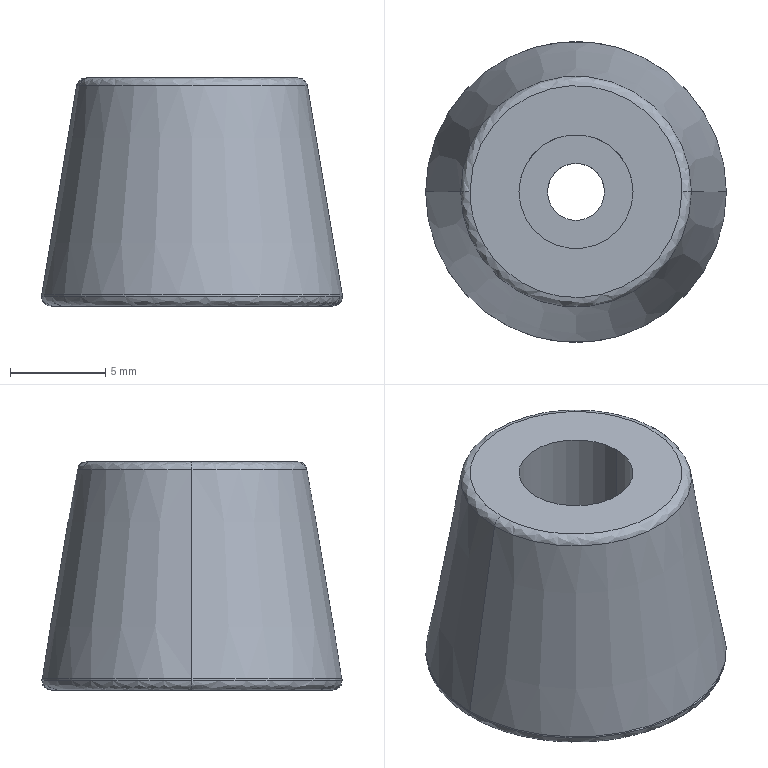Part | SolidWorks | features BaseBody 1 | 1 solid | 15 faces | box 15.82 x 15.82 x 12 mm | volume 1643 mm3 | spline 6 | cylinder 4 | plane 3 | cone 2 | commonest cylinder face diameters 3 x2 6 x2
STEP:
#1=CARTESIAN_POINT('',(-7.91,0.,0.5));
#2=VERTEX_POINT('',#1);
#3=CARTESIAN_POINT('',(7.91,0.,0.5));
#4=VERTEX_POINT('',#3);
#5=CARTESIAN_POINT('',(0.,0.,0.5));
#6=DIRECTION('',(0.,0.,1.));
#7=DIRECTION('',(1.,0.,0.));
#8=AXIS2_PLACEMENT_3D('',#5,#6,#7);
#9=CIRCLE('',#8,7.91);
#10=EDGE_CURVE('',#2,#4,#9,.T.);
#11=ORIENTED_EDGE('',*,*,#10,.F.);
#12=CARTESIAN_POINT('',(-7.41,0.,0.));
#13=VERTEX_POINT('',#12);
#14=CARTESIAN_POINT('',(-7.41,0.,0.5));
#15=DIRECTION('',(0.,-1.,0.));
#16=DIRECTION('',(-1.,0.,0.));
#17=AXIS2_PLACEMENT_3D('',#14,#15,#16);
#18=CIRCLE('',#17,0.5);
#19=EDGE_CURVE('',#2,#13,#18,.T.);
#20=ORIENTED_EDGE('',*,*,#19,.T.);
#21=CARTESIAN_POINT('',(7.41,0.,0.));
#22=VERTEX_POINT('',#21);
#23=CARTESIAN_POINT('',(-7.41,0.,0.));
#24=CARTESIAN_POINT('',(-7.41,-14.82,0.));
#25=CARTESIAN_POINT('',(7.41,-14.82,0.));
#26=CARTESIAN_POINT('',(7.41,0.,0.));
#27=(BOUNDED_CURVE()B_SPLINE_CURVE(3,(#23,#24,#25,#26),.UNSPECIFIED.,.F.,.F.)B_SPLINE_CURVE_WITH_KNOTS((4,4),(0.,1.),.UNSPECIFIED.)CURVE()GEOMETRIC_REPRESENTATION_ITEM()RATIONAL_B_SPLINE_CURVE((1.,0.3333,0.3333,1.))REPRESENTATION_ITEM(''));
#28=EDGE_CURVE('',#13,#22,#27,.T.);
#29=ORIENTED_EDGE('',*,*,#28,.T.);
#30=CARTESIAN_POINT('',(7.41,0.,0.5));
#31=DIRECTION('',(0.,1.,0.));
#32=DIRECTION('',(1.,0.,0.));
#33=AXIS2_PLACEMENT_3D('',#30,#31,#32);
#34=CIRCLE('',#33,0.5);
#35=EDGE_CURVE('',#4,#22,#34,.T.);
#36=ORIENTED_EDGE('',*,*,#35,.F.);
#37=EDGE_LOOP('',(#11,#20,#29,#36));
#38=FACE_OUTER_BOUND('',#37,.T.);
#39=CARTESIAN_POINT('',(-7.91,0.,0.5));
#40=CARTESIAN_POINT('',(-7.91,-15.82,0.5));
#41=CARTESIAN_POINT('',(7.91,-15.82,0.5));
#42=CARTESIAN_POINT('',(7.91,0.,0.5));
#43=CARTESIAN_POINT('',(-7.91,0.,0.2071));
#44=CARTESIAN_POINT('',(-7.91,-15.82,0.2071));
#45=CARTESIAN_POINT('',(7.91,-15.82,0.2071));
#46=CARTESIAN_POINT('',(7.91,0.,0.2071));
#47=CARTESIAN_POINT('',(-7.703,0.,0.));
#48=CARTESIAN_POINT('',(-7.703,-15.405,0.));
#49=CARTESIAN_POINT('',(7.703,-15.405,0.));
#50=CARTESIAN_POINT('',(7.703,0.,0.));
#51=CARTESIAN_POINT('',(-7.41,0.,0.));
#52=CARTESIAN_POINT('',(-7.41,-14.82,0.));
#53=CARTESIAN_POINT('',(7.41,-14.82,0.));
#54=CARTESIAN_POINT('',(7.41,0.,0.));
#55=(BOUNDED_SURFACE()B_SPLINE_SURFACE(3,3,((#39,#40,#41,#42),(#43,#44,#45,#46),(#47,#48,#49,#50),(#51,#52,#53,#54)),.UNSPECIFIED.,.F.,.F.,.F.)B_SPLINE_SURFACE_WITH_KNOTS((4,4),(4,4),(0.,1.),(0.,1.),.UNSPECIFIED.)GEOMETRIC_REPRESENTATION_ITEM()RATIONAL_B_SPLINE_SURFACE(((1.,0.3333,0.3333,1.),(0.8047,0.2682,0.2682,0.8047),(0.8047,0.2682,0.2682,0.8047),(1.,0.3333,0.3333,1.)))REPRESENTATION_ITEM('')SURFACE());
#56=ADVANCED_FACE('',(#38),#55,.T.);
#57=CARTESIAN_POINT('',(5.576,0.,12.));
#58=VERTEX_POINT('',#57);
#59=CARTESIAN_POINT('',(-5.576,0.,12.));
#60=VERTEX_POINT('',#59);
#61=CARTESIAN_POINT('',(5.576,0.,12.));
#62=CARTESIAN_POINT('',(5.576,-11.153,12.));
#63=CARTESIAN_POINT('',(-5.576,-11.153,12.));
#64=CARTESIAN_POINT('',(-5.576,0.,12.));
#65=(BOUNDED_CURVE()B_SPLINE_CURVE(3,(#61,#62,#63,#64),.UNSPECIFIED.,.F.,.F.)B_SPLINE_CURVE_WITH_KNOTS((4,4),(0.,1.),.UNSPECIFIED.)CURVE()GEOMETRIC_REPRESENTATION_ITEM()RATIONAL_B_SPLINE_CURVE((1.,0.3333,0.3333,1.))REPRESENTATION_ITEM(''));
#66=EDGE_CURVE('',#58,#60,#65,.T.);
#67=ORIENTED_EDGE('',*,*,#66,.T.);
#68=CARTESIAN_POINT('',(-6.07,0.,11.582));
#69=VERTEX_POINT('',#68);
#70=CARTESIAN_POINT('',(-5.576,0.,11.5));
#71=DIRECTION('',(0.,-1.,0.));
#72=DIRECTION('',(-1.,0.,0.));
#73=AXIS2_PLACEMENT_3D('',#70,#71,#72);
#74=CIRCLE('',#73,0.5);
#75=EDGE_CURVE('',#60,#69,#74,.T.);
#76=ORIENTED_EDGE('',*,*,#75,.T.);
#77=CARTESIAN_POINT('',(6.07,0.,11.582));
#78=VERTEX_POINT('',#77);
#79=CARTESIAN_POINT('',(0.,0.,11.582));
#80=DIRECTION('',(0.,0.,-1.));
#81=DIRECTION('',(-1.,0.,0.));
#82=AXIS2_PLACEMENT_3D('',#79,#80,#81);
#83=CIRCLE('',#82,6.07);
#84=EDGE_CURVE('',#78,#69,#83,.T.);
#85=ORIENTED_EDGE('',*,*,#84,.F.);
#86=CARTESIAN_POINT('',(5.576,0.,11.5));
#87=DIRECTION('',(0.,1.,0.));
#88=DIRECTION('',(1.,0.,0.));
#89=AXIS2_PLACEMENT_3D('',#86,#87,#88);
#90=CIRCLE('',#89,0.5);
#91=EDGE_CURVE('',#58,#78,#90,.T.);
#92=ORIENTED_EDGE('',*,*,#91,.F.);
#93=EDGE_LOOP('',(#67,#76,#85,#92));
#94=FACE_OUTER_BOUND('',#93,.T.);
#95=CARTESIAN_POINT('',(-5.576,0.,12.));
#96=CARTESIAN_POINT('',(-5.576,-11.153,12.));
#97=CARTESIAN_POINT('',(5.576,-11.153,12.));
#98=CARTESIAN_POINT('',(5.576,0.,12.));
#99=CARTESIAN_POINT('',(-5.832,0.,12.));
#100=CARTESIAN_POINT('',(-5.832,-11.665,12.));
#101=CARTESIAN_POINT('',(5.832,-11.665,12.));
#102=CARTESIAN_POINT('',(5.832,0.,12.));
#103=CARTESIAN_POINT('',(-6.028,0.,11.835));
#104=CARTESIAN_POINT('',(-6.028,-12.055,11.835));
#105=CARTESIAN_POINT('',(6.028,-12.055,11.835));
#106=CARTESIAN_POINT('',(6.028,0.,11.835));
#107=CARTESIAN_POINT('',(-6.07,0.,11.582));
#108=CARTESIAN_POINT('',(-6.07,-12.139,11.582));
#109=CARTESIAN_POINT('',(6.07,-12.139,11.582));
#110=CARTESIAN_POINT('',(6.07,0.,11.582));
#111=(BOUNDED_SURFACE()B_SPLINE_SURFACE(3,3,((#95,#96,#97,#98),(#99,#100,#101,#102),(#103,#104,#105,#106),(#107,#108,#109,#110)),.UNSPECIFIED.,.F.,.F.,.F.)B_SPLINE_SURFACE_WITH_KNOTS((4,4),(4,4),(0.,1.),(0.,1.),.UNSPECIFIED.)GEOMETRIC_REPRESENTATION_ITEM()RATIONAL_B_SPLINE_SURFACE(((1.,0.3333,0.3333,1.),(0.842,0.2807,0.2807,0.842),(0.842,0.2807,0.2807,0.842),(1.,0.3333,0.3333,1.)))REPRESENTATION_ITEM('')SURFACE());
#112=ADVANCED_FACE('',(#94),#111,.T.);
#113=CARTESIAN_POINT('',(-7.903,0.,0.5822));
#114=VERTEX_POINT('',#113);
#115=CARTESIAN_POINT('',(7.903,0.,0.5822));
#116=VERTEX_POINT('',#115);
#117=CARTESIAN_POINT('',(0.,0.,0.5822));
#118=DIRECTION('',(0.,0.,1.));
#119=DIRECTION('',(-1.,0.,0.));
#120=AXIS2_PLACEMENT_3D('',#117,#118,#119);
#121=CIRCLE('',#120,7.903);
#122=EDGE_CURVE('',#114,#116,#121,.T.);
#123=ORIENTED_EDGE('',*,*,#122,.F.);
#124=CARTESIAN_POINT('',(-7.41,0.,0.5));
#125=DIRECTION('',(0.,-1.,0.));
#126=DIRECTION('',(-1.,0.,0.));
#127=AXIS2_PLACEMENT_3D('',#124,#125,#126);
#128=CIRCLE('',#127,0.5);
#129=EDGE_CURVE('',#114,#2,#128,.T.);
#130=ORIENTED_EDGE('',*,*,#129,.T.);
#131=ORIENTED_EDGE('',*,*,#10,.T.);
#132=CARTESIAN_POINT('',(7.41,0.,0.5));
#133=DIRECTION('',(0.,1.,0.));
#134=DIRECTION('',(1.,0.,0.));
#135=AXIS2_PLACEMENT_3D('',#132,#133,#134);
#136=CIRCLE('',#135,0.5);
#137=EDGE_CURVE('',#116,#4,#136,.T.);
#138=ORIENTED_EDGE('',*,*,#137,.F.);
#139=EDGE_LOOP('',(#123,#130,#131,#138));
#140=FACE_OUTER_BOUND('',#139,.T.);
#141=CARTESIAN_POINT('',(-7.903,0.,0.5822));
#142=CARTESIAN_POINT('',(-7.903,-15.806,0.5822));
#143=CARTESIAN_POINT('',(7.903,-15.806,0.5822));
#144=CARTESIAN_POINT('',(7.903,0.,0.5822));
#145=CARTESIAN_POINT('',(-7.907,0.,0.555));
#146=CARTESIAN_POINT('',(-7.907,-15.815,0.555));
#147=CARTESIAN_POINT('',(7.907,-15.815,0.555));
#148=CARTESIAN_POINT('',(7.907,0.,0.555));
#149=CARTESIAN_POINT('',(-7.91,0.,0.5276));
#150=CARTESIAN_POINT('',(-7.91,-15.82,0.5276));
#151=CARTESIAN_POINT('',(7.91,-15.82,0.5276));
#152=CARTESIAN_POINT('',(7.91,0.,0.5276));
#153=CARTESIAN_POINT('',(-7.91,0.,0.5));
#154=CARTESIAN_POINT('',(-7.91,-15.82,0.5));
#155=CARTESIAN_POINT('',(7.91,-15.82,0.5));
#156=CARTESIAN_POINT('',(7.91,0.,0.5));
#157=(BOUNDED_SURFACE()B_SPLINE_SURFACE(3,3,((#141,#142,#143,#144),(#145,#146,#147,#148),(#149,#150,#151,#152),(#153,#154,#155,#156)),.UNSPECIFIED.,.F.,.F.,.F.)B_SPLINE_SURFACE_WITH_KNOTS((4,4),(4,4),(0.,1.),(0.,1.),.UNSPECIFIED.)GEOMETRIC_REPRESENTATION_ITEM()RATIONAL_B_SPLINE_SURFACE(((1.,0.3333,0.3333,1.),(0.9977,0.3326,0.3326,0.9977),(0.9977,0.3326,0.3326,0.9977),(1.,0.3333,0.3333,1.)))REPRESENTATION_ITEM('')SURFACE());
#158=ADVANCED_FACE('',(#140),#157,.T.);
#159=CARTESIAN_POINT('',(0.,0.,11.582));
#160=DIRECTION('',(0.,0.,-1.));
#161=DIRECTION('',(-1.,0.,0.));
#162=AXIS2_PLACEMENT_3D('',#159,#160,#161);
#163=CIRCLE('',#162,6.07);
#164=EDGE_CURVE('',#69,#78,#163,.T.);
#165=ORIENTED_EDGE('',*,*,#164,.T.);
#166=CARTESIAN_POINT('',(7.903,0.,0.5822));
#167=DIRECTION('',(0.1644,0.,-0.9864));
#168=VECTOR('',#167,1000.);
#169=LINE('',#166,#168);
#170=EDGE_CURVE('',#78,#116,#169,.T.);
#171=ORIENTED_EDGE('',*,*,#170,.T.);
#172=CARTESIAN_POINT('',(0.,0.,0.5822));
#173=DIRECTION('',(0.,0.,1.));
#174=DIRECTION('',(-1.,0.,0.));
#175=AXIS2_PLACEMENT_3D('',#172,#173,#174);
#176=CIRCLE('',#175,7.903);
#177=EDGE_CURVE('',#116,#114,#176,.T.);
#178=ORIENTED_EDGE('',*,*,#177,.T.);
#179=CARTESIAN_POINT('',(-7.903,0.,0.5822));
#180=DIRECTION('',(-0.1644,0.,-0.9864));
#181=VECTOR('',#180,1000.);
#182=LINE('',#179,#181);
#183=EDGE_CURVE('',#69,#114,#182,.T.);
#184=ORIENTED_EDGE('',*,*,#183,.F.);
#185=EDGE_LOOP('',(#165,#171,#178,#184));
#186=FACE_OUTER_BOUND('',#185,.T.);
#187=CARTESIAN_POINT('',(0.,0.,0.5822));
#188=DIRECTION('',(0.,0.,-1.));
#189=DIRECTION('',(-1.,0.,0.));
#190=AXIS2_PLACEMENT_3D('',#187,#188,#189);
#191=CONICAL_SURFACE('',#190,7.903,0.1651);
#192=ADVANCED_FACE('',(#186),#191,.T.);
#193=ORIENTED_EDGE('',*,*,#129,.F.);
#194=ORIENTED_EDGE('',*,*,#177,.F.);
#195=ORIENTED_EDGE('',*,*,#137,.T.);
#196=CARTESIAN_POINT('',(0.,0.,0.5));
#197=DIRECTION('',(0.,0.,1.));
#198=DIRECTION('',(1.,0.,0.));
#199=AXIS2_PLACEMENT_3D('',#196,#197,#198);
#200=CIRCLE('',#199,7.91);
#201=EDGE_CURVE('',#4,#2,#200,.T.);
#202=ORIENTED_EDGE('',*,*,#201,.T.);
#203=EDGE_LOOP('',(#193,#194,#195,#202));
#204=FACE_OUTER_BOUND('',#203,.T.);
#205=CARTESIAN_POINT('',(7.903,0.,0.5822));
#206=CARTESIAN_POINT('',(7.903,15.806,0.5822));
#207=CARTESIAN_POINT('',(-7.903,15.806,0.5822));
#208=CARTESIAN_POINT('',(-7.903,0.,0.5822));
#209=CARTESIAN_POINT('',(7.907,0.,0.555));
#210=CARTESIAN_POINT('',(7.907,15.815,0.555));
#211=CARTESIAN_POINT('',(-7.907,15.815,0.555));
#212=CARTESIAN_POINT('',(-7.907,0.,0.555));
#213=CARTESIAN_POINT('',(7.91,0.,0.5276));
#214=CARTESIAN_POINT('',(7.91,15.82,0.5276));
#215=CARTESIAN_POINT('',(-7.91,15.82,0.5276));
#216=CARTESIAN_POINT('',(-7.91,0.,0.5276));
#217=CARTESIAN_POINT('',(7.91,0.,0.5));
#218=CARTESIAN_POINT('',(7.91,15.82,0.5));
#219=CARTESIAN_POINT('',(-7.91,15.82,0.5));
#220=CARTESIAN_POINT('',(-7.91,0.,0.5));
#221=(BOUNDED_SURFACE()B_SPLINE_SURFACE(3,3,((#205,#206,#207,#208),(#209,#210,#211,#212),(#213,#214,#215,#216),(#217,#218,#219,#220)),.UNSPECIFIED.,.F.,.F.,.F.)B_SPLINE_SURFACE_WITH_KNOTS((4,4),(4,4),(0.,1.),(0.,1.),.UNSPECIFIED.)GEOMETRIC_REPRESENTATION_ITEM()RATIONAL_B_SPLINE_SURFACE(((1.,0.3333,0.3333,1.),(0.9977,0.3326,0.3326,0.9977),(0.9977,0.3326,0.3326,0.9977),(1.,0.3333,0.3333,1.)))REPRESENTATION_ITEM('')SURFACE());
#222=ADVANCED_FACE('',(#204),#221,.T.);
#223=CARTESIAN_POINT('',(1.5,0.,6.));
#224=VERTEX_POINT('',#223);
#225=CARTESIAN_POINT('',(-1.5,0.,6.));
#226=VERTEX_POINT('',#225);
#227=CARTESIAN_POINT('',(0.,0.,6.));
#228=DIRECTION('',(0.,0.,-1.));
#229=DIRECTION('',(-1.,0.,0.));
#230=AXIS2_PLACEMENT_3D('',#227,#228,#229);
#231=CIRCLE('',#230,1.5);
#232=EDGE_CURVE('',#224,#226,#231,.T.);
#233=ORIENTED_EDGE('',*,*,#232,.F.);
#234=CARTESIAN_POINT('',(1.5,0.,0.));
#235=VERTEX_POINT('',#234);
#236=CARTESIAN_POINT('',(1.5,0.,12.));
#237=DIRECTION('',(0.,0.,-1.));
#238=VECTOR('',#237,1000.);
#239=LINE('',#236,#238);
#240=EDGE_CURVE('',#224,#235,#239,.T.);
#241=ORIENTED_EDGE('',*,*,#240,.T.);
#242=CARTESIAN_POINT('',(-1.5,0.,0.));
#243=VERTEX_POINT('',#242);
#244=CARTESIAN_POINT('',(0.,0.,0.));
#245=DIRECTION('',(0.,0.,-1.));
#246=DIRECTION('',(-1.,0.,0.));
#247=AXIS2_PLACEMENT_3D('',#244,#245,#246);
#248=CIRCLE('',#247,1.5);
#249=EDGE_CURVE('',#235,#243,#248,.T.);
#250=ORIENTED_EDGE('',*,*,#249,.T.);
#251=CARTESIAN_POINT('',(-1.5,0.,12.));
#252=DIRECTION('',(0.,0.,-1.));
#253=VECTOR('',#252,1000.);
#254=LINE('',#251,#253);
#255=EDGE_CURVE('',#226,#243,#254,.T.);
#256=ORIENTED_EDGE('',*,*,#255,.F.);
#257=EDGE_LOOP('',(#233,#241,#250,#256));
#258=FACE_OUTER_BOUND('',#257,.T.);
#259=CARTESIAN_POINT('',(0.,0.,12.));
#260=DIRECTION('',(0.,0.,-1.));
#261=DIRECTION('',(-1.,0.,0.));
#262=AXIS2_PLACEMENT_3D('',#259,#260,#261);
#263=CYLINDRICAL_SURFACE('',#262,1.5);
#264=ADVANCED_FACE('',(#258),#263,.F.);
#265=CARTESIAN_POINT('',(-3.,0.,6.));
#266=VERTEX_POINT('',#265);
#267=CARTESIAN_POINT('',(3.,0.,6.));
#268=VERTEX_POINT('',#267);
#269=CARTESIAN_POINT('',(0.,0.,6.));
#270=DIRECTION('',(0.,0.,1.));
#271=DIRECTION('',(1.,0.,0.));
#272=AXIS2_PLACEMENT_3D('',#269,#270,#271);
#273=CIRCLE('',#272,3.);
#274=EDGE_CURVE('',#266,#268,#273,.T.);
#275=ORIENTED_EDGE('',*,*,#274,.F.);
#276=CARTESIAN_POINT('',(-3.,0.,12.));
#277=VERTEX_POINT('',#276);
#278=CARTESIAN_POINT('',(-3.,0.,6.));
#279=DIRECTION('',(0.,0.,1.));
#280=VECTOR('',#279,1000.);
#281=LINE('',#278,#280);
#282=EDGE_CURVE('',#266,#277,#281,.T.);
#283=ORIENTED_EDGE('',*,*,#282,.T.);
#284=CARTESIAN_POINT('',(3.,0.,12.));
#285=VERTEX_POINT('',#284);
#286=CARTESIAN_POINT('',(0.,0.,12.));
#287=DIRECTION('',(0.,0.,-1.));
#288=DIRECTION('',(1.,0.,0.));
#289=AXIS2_PLACEMENT_3D('',#286,#287,#288);
#290=CIRCLE('',#289,3.);
#291=EDGE_CURVE('',#285,#277,#290,.T.);
#292=ORIENTED_EDGE('',*,*,#291,.F.);
#293=CARTESIAN_POINT('',(3.,0.,6.));
#294=DIRECTION('',(0.,0.,1.));
#295=VECTOR('',#294,1000.);
#296=LINE('',#293,#295);
#297=EDGE_CURVE('',#268,#285,#296,.T.);
#298=ORIENTED_EDGE('',*,*,#297,.F.);
#299=EDGE_LOOP('',(#275,#283,#292,#298));
#300=FACE_OUTER_BOUND('',#299,.T.);
#301=CARTESIAN_POINT('',(0.,0.,6.));
#302=DIRECTION('',(0.,0.,1.));
#303=DIRECTION('',(1.,0.,0.));
#304=AXIS2_PLACEMENT_3D('',#301,#302,#303);
#305=CYLINDRICAL_SURFACE('',#304,3.);
#306=ADVANCED_FACE('',(#300),#305,.F.);
#307=ORIENTED_EDGE('',*,*,#170,.F.);
#308=ORIENTED_EDGE('',*,*,#84,.T.);
#309=ORIENTED_EDGE('',*,*,#183,.T.);
#310=ORIENTED_EDGE('',*,*,#122,.T.);
#311=EDGE_LOOP('',(#307,#308,#309,#310));
#312=FACE_OUTER_BOUND('',#311,.T.);
#313=CARTESIAN_POINT('',(0.,0.,0.5822));
#314=DIRECTION('',(0.,0.,-1.));
#315=DIRECTION('',(-1.,0.,0.));
#316=AXIS2_PLACEMENT_3D('',#313,#314,#315);
#317=CONICAL_SURFACE('',#316,7.903,0.1651);
#318=ADVANCED_FACE('',(#312),#317,.T.);
#319=ORIENTED_EDGE('',*,*,#19,.F.);
#320=ORIENTED_EDGE('',*,*,#201,.F.);
#321=ORIENTED_EDGE('',*,*,#35,.T.);
#322=CARTESIAN_POINT('',(7.41,0.,0.));
#323=CARTESIAN_POINT('',(7.41,14.82,0.));
#324=CARTESIAN_POINT('',(-7.41,14.82,0.));
#325=CARTESIAN_POINT('',(-7.41,0.,0.));
#326=(BOUNDED_CURVE()B_SPLINE_CURVE(3,(#322,#323,#324,#325),.UNSPECIFIED.,.F.,.F.)B_SPLINE_CURVE_WITH_KNOTS((4,4),(0.,1.),.UNSPECIFIED.)CURVE()GEOMETRIC_REPRESENTATION_ITEM()RATIONAL_B_SPLINE_CURVE((1.,0.3333,0.3333,1.))REPRESENTATION_ITEM(''));
#327=EDGE_CURVE('',#22,#13,#326,.T.);
#328=ORIENTED_EDGE('',*,*,#327,.T.);
#329=EDGE_LOOP('',(#319,#320,#321,#328));
#330=FACE_OUTER_BOUND('',#329,.T.);
#331=CARTESIAN_POINT('',(7.91,0.,0.5));
#332=CARTESIAN_POINT('',(7.91,15.82,0.5));
#333=CARTESIAN_POINT('',(-7.91,15.82,0.5));
#334=CARTESIAN_POINT('',(-7.91,0.,0.5));
#335=CARTESIAN_POINT('',(7.91,0.,0.2071));
#336=CARTESIAN_POINT('',(7.91,15.82,0.2071));
#337=CARTESIAN_POINT('',(-7.91,15.82,0.2071));
#338=CARTESIAN_POINT('',(-7.91,0.,0.2071));
#339=CARTESIAN_POINT('',(7.703,0.,0.));
#340=CARTESIAN_POINT('',(7.703,15.405,0.));
#341=CARTESIAN_POINT('',(-7.703,15.405,0.));
#342=CARTESIAN_POINT('',(-7.703,0.,0.));
#343=CARTESIAN_POINT('',(7.41,0.,0.));
#344=CARTESIAN_POINT('',(7.41,14.82,0.));
#345=CARTESIAN_POINT('',(-7.41,14.82,0.));
#346=CARTESIAN_POINT('',(-7.41,0.,0.));
#347=(BOUNDED_SURFACE()B_SPLINE_SURFACE(3,3,((#331,#332,#333,#334),(#335,#336,#337,#338),(#339,#340,#341,#342),(#343,#344,#345,#346)),.UNSPECIFIED.,.F.,.F.,.F.)B_SPLINE_SURFACE_WITH_KNOTS((4,4),(4,4),(0.,1.),(0.,1.),.UNSPECIFIED.)GEOMETRIC_REPRESENTATION_ITEM()RATIONAL_B_SPLINE_SURFACE(((1.,0.3333,0.3333,1.),(0.8047,0.2682,0.2682,0.8047),(0.8047,0.2682,0.2682,0.8047),(1.,0.3333,0.3333,1.)))REPRESENTATION_ITEM('')SURFACE());
#348=ADVANCED_FACE('',(#330),#347,.T.);
#349=ORIENTED_EDGE('',*,*,#75,.F.);
#350=CARTESIAN_POINT('',(-5.576,0.,12.));
#351=CARTESIAN_POINT('',(-5.576,11.153,12.));
#352=CARTESIAN_POINT('',(5.576,11.153,12.));
#353=CARTESIAN_POINT('',(5.576,0.,12.));
#354=(BOUNDED_CURVE()B_SPLINE_CURVE(3,(#350,#351,#352,#353),.UNSPECIFIED.,.F.,.F.)B_SPLINE_CURVE_WITH_KNOTS((4,4),(0.,1.),.UNSPECIFIED.)CURVE()GEOMETRIC_REPRESENTATION_ITEM()RATIONAL_B_SPLINE_CURVE((1.,0.3333,0.3333,1.))REPRESENTATION_ITEM(''));
#355=EDGE_CURVE('',#60,#58,#354,.T.);
#356=ORIENTED_EDGE('',*,*,#355,.T.);
#357=ORIENTED_EDGE('',*,*,#91,.T.);
#358=ORIENTED_EDGE('',*,*,#164,.F.);
#359=EDGE_LOOP('',(#349,#356,#357,#358));
#360=FACE_OUTER_BOUND('',#359,.T.);
#361=CARTESIAN_POINT('',(5.576,0.,12.));
#362=CARTESIAN_POINT('',(5.576,11.153,12.));
#363=CARTESIAN_POINT('',(-5.576,11.153,12.));
#364=CARTESIAN_POINT('',(-5.576,0.,12.));
#365=CARTESIAN_POINT('',(5.832,0.,12.));
#366=CARTESIAN_POINT('',(5.832,11.665,12.));
#367=CARTESIAN_POINT('',(-5.832,11.665,12.));
#368=CARTESIAN_POINT('',(-5.832,0.,12.));
#369=CARTESIAN_POINT('',(6.028,0.,11.835));
#370=CARTESIAN_POINT('',(6.028,12.055,11.835));
#371=CARTESIAN_POINT('',(-6.028,12.055,11.835));
#372=CARTESIAN_POINT('',(-6.028,0.,11.835));
#373=CARTESIAN_POINT('',(6.07,0.,11.582));
#374=CARTESIAN_POINT('',(6.07,12.139,11.582));
#375=CARTESIAN_POINT('',(-6.07,12.139,11.582));
#376=CARTESIAN_POINT('',(-6.07,0.,11.582));
#377=(BOUNDED_SURFACE()B_SPLINE_SURFACE(3,3,((#361,#362,#363,#364),(#365,#366,#367,#368),(#369,#370,#371,#372),(#373,#374,#375,#376)),.UNSPECIFIED.,.F.,.F.,.F.)B_SPLINE_SURFACE_WITH_KNOTS((4,4),(4,4),(0.,1.),(0.,1.),.UNSPECIFIED.)GEOMETRIC_REPRESENTATION_ITEM()RATIONAL_B_SPLINE_SURFACE(((1.,0.3333,0.3333,1.),(0.842,0.2807,0.2807,0.842),(0.842,0.2807,0.2807,0.842),(1.,0.3333,0.3333,1.)))REPRESENTATION_ITEM('')SURFACE());
#378=ADVANCED_FACE('',(#360),#377,.T.);
#379=CARTESIAN_POINT('',(0.,0.,0.));
#380=DIRECTION('',(0.,0.,-1.));
#381=DIRECTION('',(-1.,0.,0.));
#382=AXIS2_PLACEMENT_3D('',#379,#380,#381);
#383=CIRCLE('',#382,1.5);
#384=EDGE_CURVE('',#243,#235,#383,.T.);
#385=ORIENTED_EDGE('',*,*,#384,.F.);
#386=ORIENTED_EDGE('',*,*,#249,.F.);
#387=EDGE_LOOP('',(#385,#386));
#388=FACE_BOUND('',#387,.T.);
#389=ORIENTED_EDGE('',*,*,#327,.F.);
#390=ORIENTED_EDGE('',*,*,#28,.F.);
#391=EDGE_LOOP('',(#389,#390));
#392=FACE_OUTER_BOUND('',#391,.T.);
#393=CARTESIAN_POINT('',(0.,0.,0.));
#394=DIRECTION('',(0.,0.,1.));
#395=DIRECTION('',(1.,0.,0.));
#396=AXIS2_PLACEMENT_3D('',#393,#394,#395);
#397=PLANE('',#396);
#398=ADVANCED_FACE('',(#388,#392),#397,.F.);
#399=ORIENTED_EDGE('',*,*,#291,.T.);
#400=CARTESIAN_POINT('',(0.,0.,12.));
#401=DIRECTION('',(0.,0.,-1.));
#402=DIRECTION('',(1.,0.,0.));
#403=AXIS2_PLACEMENT_3D('',#400,#401,#402);
#404=CIRCLE('',#403,3.);
#405=EDGE_CURVE('',#277,#285,#404,.T.);
#406=ORIENTED_EDGE('',*,*,#405,.T.);
#407=EDGE_LOOP('',(#399,#406));
#408=FACE_BOUND('',#407,.T.);
#409=ORIENTED_EDGE('',*,*,#355,.F.);
#410=ORIENTED_EDGE('',*,*,#66,.F.);
#411=EDGE_LOOP('',(#409,#410));
#412=FACE_OUTER_BOUND('',#411,.T.);
#413=CARTESIAN_POINT('',(0.,0.,12.));
#414=DIRECTION('',(0.,0.,1.));
#415=DIRECTION('',(1.,0.,0.));
#416=AXIS2_PLACEMENT_3D('',#413,#414,#415);
#417=PLANE('',#416);
#418=ADVANCED_FACE('',(#408,#412),#417,.T.);
#419=ORIENTED_EDGE('',*,*,#240,.F.);
#420=CARTESIAN_POINT('',(0.,0.,6.));
#421=DIRECTION('',(0.,0.,-1.));
#422=DIRECTION('',(-1.,0.,0.));
#423=AXIS2_PLACEMENT_3D('',#420,#421,#422);
#424=CIRCLE('',#423,1.5);
#425=EDGE_CURVE('',#226,#224,#424,.T.);
#426=ORIENTED_EDGE('',*,*,#425,.F.);
#427=ORIENTED_EDGE('',*,*,#255,.T.);
#428=ORIENTED_EDGE('',*,*,#384,.T.);
#429=EDGE_LOOP('',(#419,#426,#427,#428));
#430=FACE_OUTER_BOUND('',#429,.T.);
#431=CARTESIAN_POINT('',(0.,0.,12.));
#432=DIRECTION('',(0.,0.,-1.));
#433=DIRECTION('',(-1.,0.,0.));
#434=AXIS2_PLACEMENT_3D('',#431,#432,#433);
#435=CYLINDRICAL_SURFACE('',#434,1.5);
#436=ADVANCED_FACE('',(#430),#435,.F.);
#437=ORIENTED_EDGE('',*,*,#282,.F.);
#438=CARTESIAN_POINT('',(0.,0.,6.));
#439=DIRECTION('',(0.,0.,1.));
#440=DIRECTION('',(1.,0.,0.));
#441=AXIS2_PLACEMENT_3D('',#438,#439,#440);
#442=CIRCLE('',#441,3.);
#443=EDGE_CURVE('',#268,#266,#442,.T.);
#444=ORIENTED_EDGE('',*,*,#443,.F.);
#445=ORIENTED_EDGE('',*,*,#297,.T.);
#446=ORIENTED_EDGE('',*,*,#405,.F.);
#447=EDGE_LOOP('',(#437,#444,#445,#446));
#448=FACE_OUTER_BOUND('',#447,.T.);
#449=CARTESIAN_POINT('',(0.,0.,6.));
#450=DIRECTION('',(0.,0.,1.));
#451=DIRECTION('',(1.,0.,0.));
#452=AXIS2_PLACEMENT_3D('',#449,#450,#451);
#453=CYLINDRICAL_SURFACE('',#452,3.);
#454=ADVANCED_FACE('',(#448),#453,.F.);
#455=ORIENTED_EDGE('',*,*,#443,.T.);
#456=ORIENTED_EDGE('',*,*,#274,.T.);
#457=EDGE_LOOP('',(#455,#456));
#458=FACE_OUTER_BOUND('',#457,.T.);
#459=ORIENTED_EDGE('',*,*,#425,.T.);
#460=ORIENTED_EDGE('',*,*,#232,.T.);
#461=EDGE_LOOP('',(#459,#460));
#462=FACE_BOUND('',#461,.T.);
#463=CARTESIAN_POINT('',(0.,0.,6.));
#464=DIRECTION('',(0.,0.,1.));
#465=DIRECTION('',(1.,0.,0.));
#466=AXIS2_PLACEMENT_3D('',#463,#464,#465);
#467=PLANE('',#466);
#468=ADVANCED_FACE('',(#458,#462),#467,.T.);
#469=CLOSED_SHELL('',(#56,#112,#158,#192,#222,#264,#306,#318,#348,#378,#398,#418,#436,#454,#468));
#470=MANIFOLD_SOLID_BREP('',#469);
#471=CARTESIAN_POINT('',(0.,0.,0.));
#472=DIRECTION('',(0.,0.,1.));
#473=DIRECTION('',(1.,0.,0.));
#474=AXIS2_PLACEMENT_3D('',#471,#472,#473);
#475=(LENGTH_UNIT()NAMED_UNIT(*)SI_UNIT(.MILLI.,.METRE.));
#476=UNCERTAINTY_MEASURE_WITH_UNIT(LENGTH_MEASURE(0.00001),#475,'','');
#477=(NAMED_UNIT(*)PLANE_ANGLE_UNIT()SI_UNIT($,.RADIAN.));
#478=(NAMED_UNIT(*)SI_UNIT($,.STERADIAN.)SOLID_ANGLE_UNIT());
#479=(GEOMETRIC_REPRESENTATION_CONTEXT(3)GLOBAL_UNCERTAINTY_ASSIGNED_CONTEXT((#476))GLOBAL_UNIT_ASSIGNED_CONTEXT((#475,#477,#478))REPRESENTATION_CONTEXT('',''));
#480=ADVANCED_BREP_SHAPE_REPRESENTATION('',(#470,#474),#479);